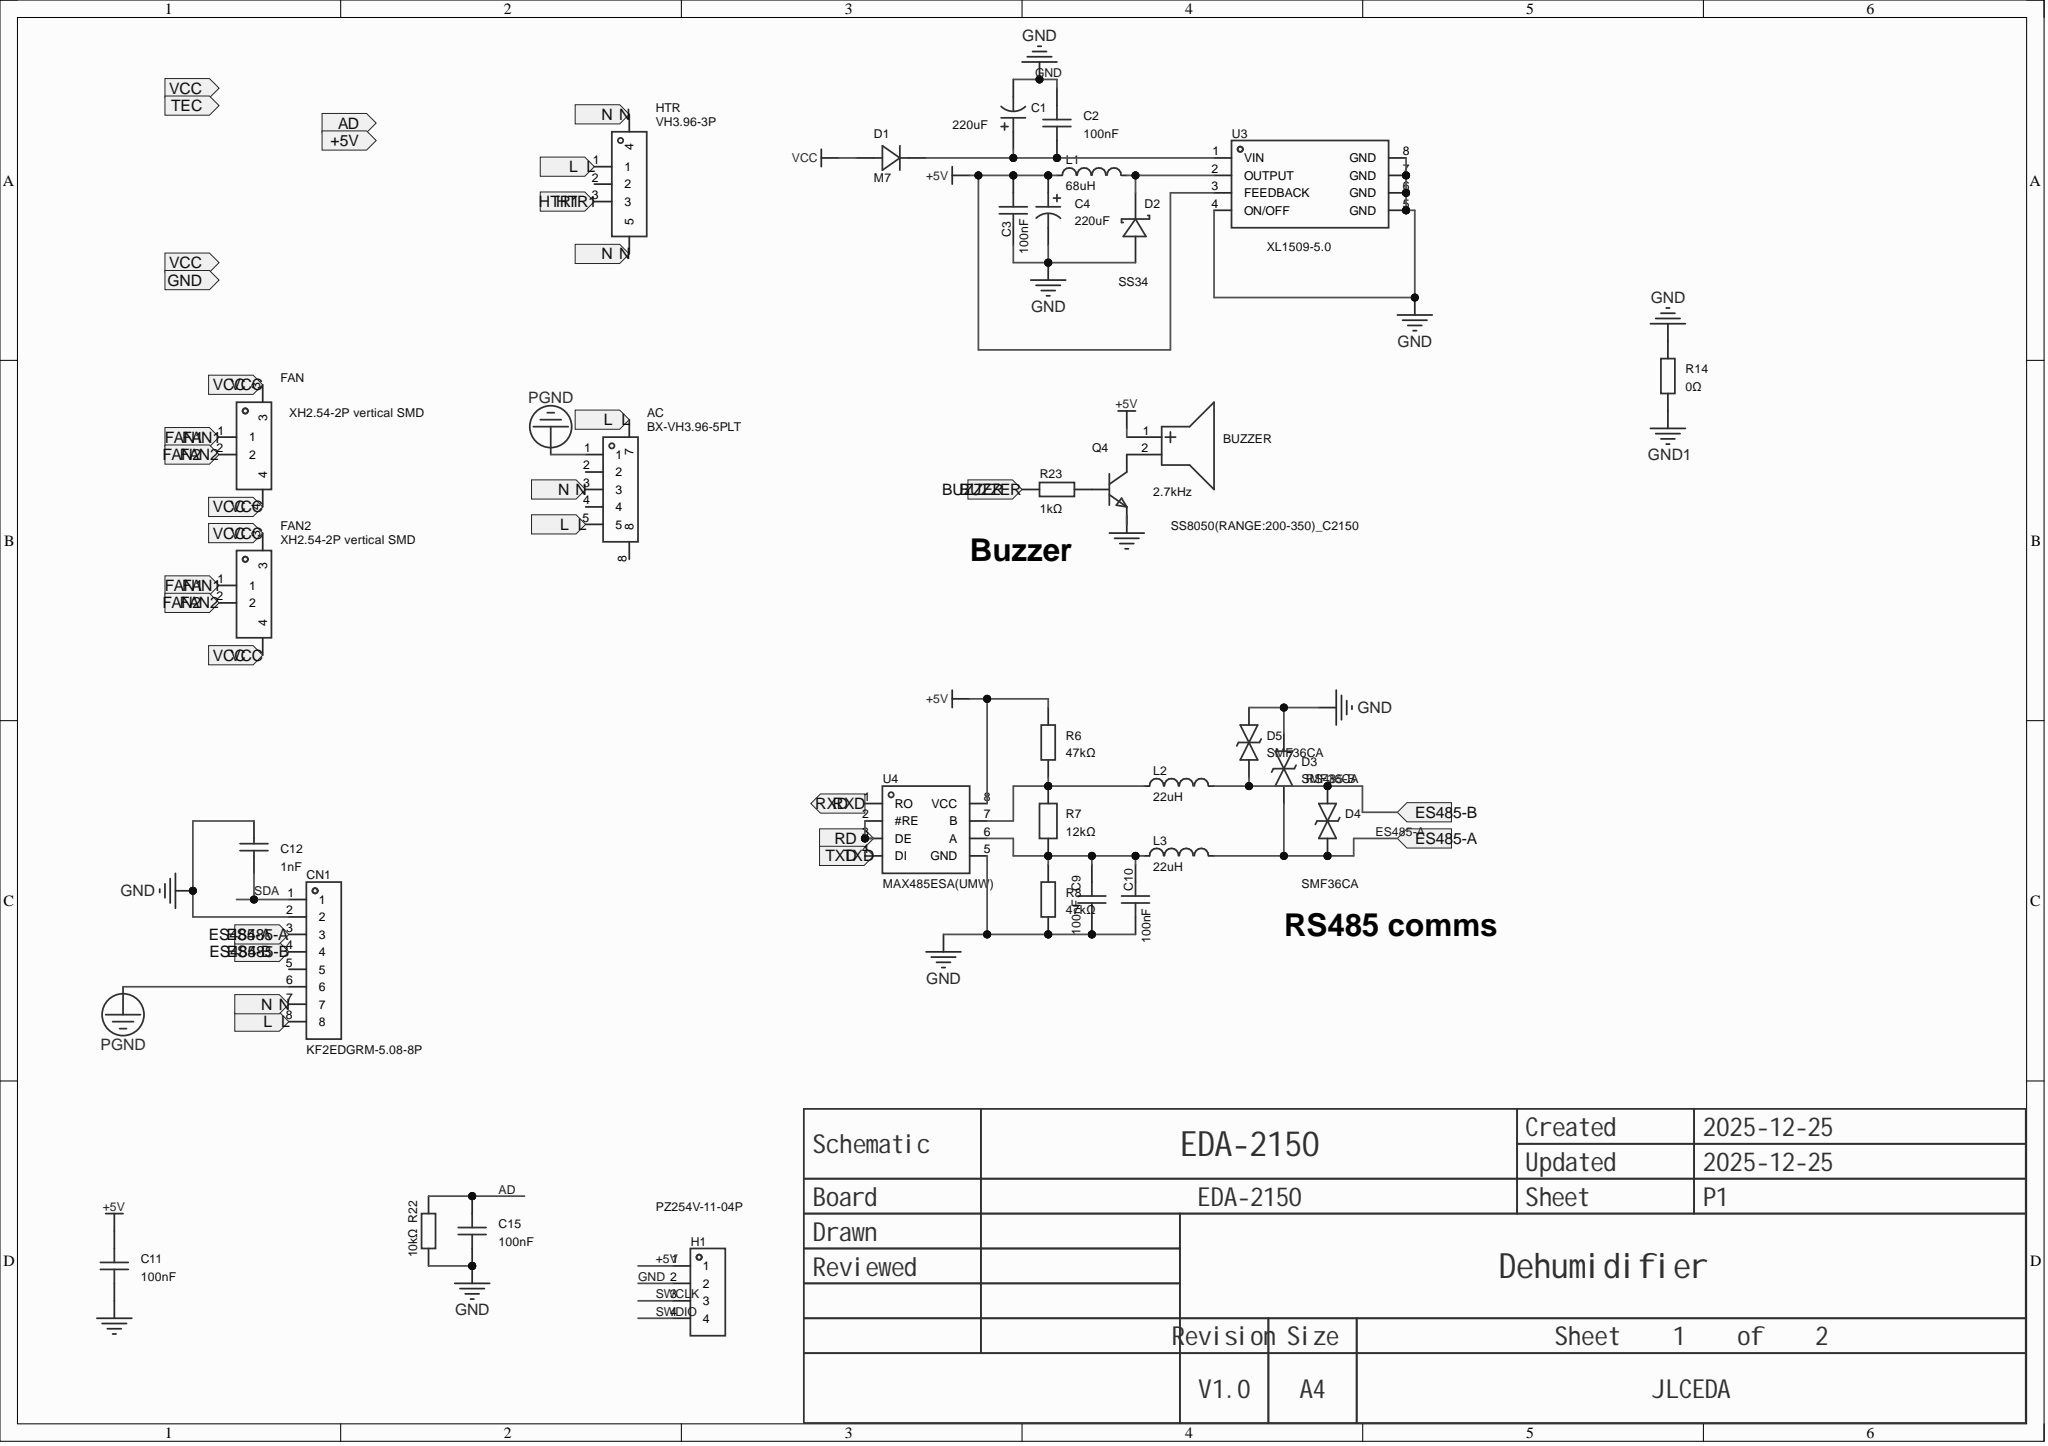Circuit board | Altium Designer | 76 parts | 60 nets
Bill of materials:
Comment,Description,Designator,Footprint,LibRef,Quantity
"BX-VH3.96-5PLT","Pin structure:1x5P;Pitch:3.96mm;Mounting:Vertical SMD;Series:VH;Total pins:5P;Rows:1;Pins per row:5;Row spacing:-;Rated current:7A;Contact material:Brass;Contact plating:Tin;Operating temp:-25℃~+85℃;","AC","CONN-SMD_5P-P3.96_BX-VH3.96-5PLT","BX-VH3.96-5PLT","1"
"2.7kHz","Drive:Active(built-in driver circuit);Frequency:2.7kHz;Sound pressure(SPL):80dB;","BUZZER","BUZ-SMD_L9.6-W9.6-LS10.0-R","YS-SBZ9650DYB05","1"
"220uF","Capacitance:220uF;Tolerance:±20%;Rated voltage:35V;Ripple current:190mA@120Hz;","C1, C4","CAP-SMD_BD6.3-L6.6-W6.6-FD","JVJ35V220M6x8","2"
"100nF","Capacitance:100nF;Tolerance:±10%;Rated voltage:50V;Temp coefficient:X7R;","C2, C3, C5, C9, C10, C11, C15, C16","C0805","FCC0805B104K500DT","8"
"100pF","Capacitance:100pF;Tolerance:±5%;Rated voltage:50V;Temp coefficient:C0G;","C6, C7, C8","C0805","CL21C101JBANNNC","3"
"1nF","Capacitance:1nF;Tolerance:±10%;Rated voltage:50V;Temp coefficient:X7R;","C12","C0805","CL21B102KBCNNNC","1"
"10nF","Capacitance:10nF;Tolerance:±10%;Rated voltage:50V;Temp coefficient:X7R;","C17","C1210","1210B103K500NT","1"
"KF2EDGRM-5.08-8P","Connector type:Board-side socket, closed;Fixing:Screw;Structure:1x8P;Pitch:5.08mm;Colour:Green;Mounting:Right-angle THT;Rows:1;Pins per row:8;Rated current:15A;Rated voltage:300V;Operating temp:-40℃~+105℃;","CN1","CONN-TH_8P-P5.08_KF2EDGRM-5.08-8P","KF2EDGRM-5.08-8P","1"
"M7","Diode configuration:1 single;Forward voltage(Vf):1.1V@1A;DC reverse voltage(Vr):1kV;Rectified current:1A;","D1","SMA_L4.4-W2.8-LS5.4-RD","M7_C46598121","1"
"SS34","Diode configuration:Single;Forward voltage(Vf):550mV@3A;DC reverse voltage(Vr):40V;Rectified current:3A;","D2, D6, D7","SMA_L4.3-W2.6-LS5.2-RD","SS34_C8678","3"
"SMF36CA","Polarity:Bidirectional;Reverse standoff voltage(Vrwm):36V;Clamping voltage:58.1V;Peak pulse current(Ipp):3.5A;Peak pulse power(Ppp):200W@10/1000us;Breakdown voltage:40V;","D3, D4, D5","SOD-123_L2.7-W1.8-LS3.7-BI","SMF36CA_C435502","3"
"XH2.54-2P vertical SMD","","FAN, FAN2","CONN-SMD_2P_A2501WV-S","XH2.54-2P立贴","2"
"PZ254V-11-04P","Pin structure:1x4P;Pitch:2.54mm;Row spacing:-;Round/square pin:Square pin;Mounting:Through-hole;Rows:Single row;Total pins:4P;Rated current:3A;Rated voltage:250V;Mating pin length:6mm;Body height:2.5mm;Tail length:3mm;Contact material:-;Operating temp:-40℃~+105℃;Colour:Black;","H1","HDR-TH_4P-P2.54-V-M","PZ254V-11-04P","1"
"VH3.96-3P","","HTR","CONN-SMD_3P-P3.96_HCTL_HC-VH-3ALT","VH3.96-3P","1"
"68uH","Inductance:68uH;Tolerance:±20%;Rated current:1.5A;Saturation current(Isat):2A;Type:-;","L1","IND-SMD_L7.1-W6.6_H5.0","PSPMAA0605H-680M-IGF","1"
"22uH","Inductance:22uH;Tolerance:±10%;Rated current:5mA;Saturation current(Isat):-;DC resistance(DCR):900mΩ;","L2, L3","L1206","SCL3216T220KSP","2"
"3mmFIR","","LED1, LED2, LED3, LED4","LED-TH_BD3.0-P2.54-FD","3mmFIR","4"
"SP420361N","Same display size as the 30V tester I bought, Digits:3 digits;Emitting colour:Red;LED polarity:Common cathode;Character height (inch):0.36;","LED5, LED6","LED-SEG-TH_SP420361N","EPHB_SP420361N 0.36英寸3位红色数码管","2"
"HYG140N10","Type:1 N-channel;Drain-source voltage(Vdss):100V;Continuous drain current(Id):45A;On-resistance(RDS(on)@Vgs,Id):-;Power(Pd):3W;Threshold voltage(Vgs(th)@Id):2.5V@250uA;","Q1","TO-252-3_L6.6-W6.1-P4.58-LS10.1-BR","NCE0140K2-VB","1"
"HYG025N06LS1B","Quantity:1 N-channel;Drain-source voltage(Vdss):60V;Continuous drain current(Id):160A;On-resistance(RDS(on)):3.3mΩ@10V;Power dissipation(Pd):125W;Threshold voltage(Vgs(th)):3V@250uA;","Q2","TO-263-2_L10.2-W8.7-P5.08-LS15.1-BR","HYG025N06LS1B","1"
"BTA216B-600D-JSM","Holding current(Ih):25mA;Off-state peak voltage(Vdrm):600V;Gate trigger current(Igt):50mA;","Q3","TO-263-3_L10.2-W9.2-P5.08-LS15.4-BR","BTA216B-600D-JSM","1"
"SS8050(RANGE:200-350)","Transistor type:NPN;Collector current(Ic):1.5A;C-E breakdown voltage(Vceo):25V;Power(Pd):300mW;DC current gain(hFE@Ic,Vce):200@800mA,1V;","Q4, Q5, Q6","SOT-23-3_L2.9-W1.3-P1.90-LS2.4-BR","SS8050(RANGE:200-350)_C2150","3"
"LBC807-25","Transistor type:PNP;Collector current(Ic):500mA;C-E breakdown voltage(Vceo):45V;Power(Pd):225mW;DC current gain(hFE@Ic,Vce):160@100mA,1.0V;","Q7","SOT-23-3_L2.9-W1.6-P1.90-LS2.8-BR","LBC807-25LT1G","1"
"1K","Resistor type:Thick film resistor;Resistance:1kΩ;Tolerance:±1%;Power:125mW;Max operating voltage:150V;Temp coefficient:±100ppm/?;","R1","R0805","0805W8F1001T5E","1"
"10kΩ","Resistor type:Thick film resistor;Resistance:1kΩ;Tolerance:±1%;Power:125mW;Max operating voltage:150V;Temp coefficient:±100ppm/?;, Resistor type:Thick film resistor;Resistance:10kΩ;Tolerance:±1%;Power:125mW;Operating voltage:150V;Temp coefficient:±100ppm/?;","R2, R3, R4, R5, R10, R17, R22","R0805","0805W8F1001T5E, 0805W8F1002T5E_C17414","7"
"47kΩ","Resistor type:Thick film resistor;Resistance:47kΩ;Tolerance:±1%;Power:125mW;Max operating voltage:150V;Temp coefficient:±100ppm/?;","R6, R8","R0805","0805W8F4702T5E","2"
"12kΩ","Resistor type:Thick film resistor;Resistance:12kΩ;Tolerance:±1%;Power:125mW;Operating voltage:150V;Temp coefficient:±100ppm/?;","R7","R0805","FRC0805F1202TS","1"
"10","","R9","R0805","Res_0805","1"
"1Ω","Resistor type:Thick film resistor;Resistance:1Ω;Tolerance:±1%;Power:250mW;Operating voltage:200V;Temp coefficient:±200ppm/?;","R11","R1206","FRC1206F1R00TS","1"
"1kΩ","Resistor type:Thick film resistor;Resistance:1kΩ;Tolerance:±1%;Power:125mW;Max operating voltage:150V;Temp coefficient:±100ppm/?;","R12, R16, R23","R0805","0805W8F1001T5E","3"
"47Ω","Resistance:47Ω;Tolerance:±0.5%;Temp coefficient:±25ppm/?;","R13","R0805","TRC0805D47R0P0525Z","1"
"0Ω","","R14","R0603","Res_0603","1"
"2.2kΩ","Resistor type:Thick film resistor;Resistance:2.2kΩ;Tolerance:±1%;Power:125mW;Operating voltage:150V;Temp coefficient:±100ppm/?;","R18","R0805","0805W8F2201T5E","1"
"51Ω","Resistor type:Thin film resistor;Resistance:51Ω;Tolerance:±1%;Power:400mW;Operating voltage:200V;Temp coefficient:±50ppm/?;","R19","R0204","MMA02040C5109FB300","1"
"150Ω","Resistor type:Thin film resistor;Resistance:150Ω;Tolerance:±0.1%;Power:250mW;Operating voltage:200V;Temp coefficient:±15ppm/?;","R20","R0204","MMA02040E1500BB100","1"
"120Ω","Resistance:120Ω;Tolerance:±1%;Power:250mW;Temp coefficient:±50ppm/?;","R21","R0204","CSR0204FTDV1200","1"
"1TS005F-2500-5001","Circuit:SPST;Button shape:Round button;Actuation force:2.5N;Mounting:Vertical SMD;Switch length:6mm;Switch width:6mm;Switch height:5mm;Bracket:Without bracket;Contact current:50mA;Rated voltage:12V;Lamp:None;Life:7 ten-thousand cycles;","SW1, SW2, SW3, SW4","SW-SMD_4P-L6.0-W6.0-P4.50-LS9.0-H2.5","1TS005F-2500-5001","4"
"TSSOP-20","","U1","TSSOP-20_L6.5-W4.4-P0.65-LS6.4-BL","LCM08F003","1"
"XL1509-5.0","Function:Buck;Output type:Fixed;Operating voltage:4.5V~40V;Output voltage:5V;Output current:2A;","U3","SOIC-8_L4.9-W3.9-P1.27-LS6.0-TR","XL1509-5.0","1"
"MAX485ESA(UMW)","","U4","SOP-8_L5.0-W4.0-P1.27-LS6.0-BL","MAX485ESA(UMW)","1"
"ELM3083(TA)-V","Forward voltage:1.5V;Forward current:60mA;Load voltage:800V;Static dv/dt:1000V/us;","U5","SOP-4_L4.4-W4.0-P2.54-LS7.0-TL","ELM3083(TA)-V","1"
"TM1668-SSOP24-TA2108","Type:-;Operating voltage(DC):3V~6V;Switching frequency:-;Channels:-;Output voltage:-;Output current:-;Dimming:-;Topology:-;","U6","SSOP-24_L8.1-W5.3-P0.65-LS7.8-BL","TM1668-SSOP24-TA2108","1"
Netlist (Protel format):
[
AC
CONN-SMD_5P-P3.96_BX-VH3.96-5PLT
BX-VH3.96-5PLT



]
[
BUZZER
BUZ-SMD_L9.6-W9.6-LS10.0-R
2.7kHz



]
[
C1
CAP-SMD_BD6.3-L6.6-W6.6-FD
220uF



]
[
C2
C0805
100nF



]
[
C3
C0805
100nF



]
[
C4
CAP-SMD_BD6.3-L6.6-W6.6-FD
220uF



]
[
C5
C0805
100nF



]
[
C6
C0805
100pF



]
[
C7
C0805
100pF



]
[
C8
C0805
100pF



]
[
C9
C0805
100nF



]
[
C10
C0805
100nF



]
[
C11
C0805
100nF



]
[
C12
C0805
1nF



]
[
C15
C0805
100nF



]
[
C16
C0805
100nF



]
[
C17
C1210
10nF



]
[
CN1
CONN-TH_8P-P5.08_KF2EDGRM-5.08-8P
KF2EDGRM-5.08-8P



]
[
D1
SMA_L4.4-W2.8-LS5.4-RD
M7



]
[
D2
SMA_L4.3-W2.6-LS5.2-RD
SS34



]
[
D3
SOD-123_L2.7-W1.8-LS3.7-BI
SMF36CA



]
[
D4
SOD-123_L2.7-W1.8-LS3.7-BI
SMF36CA



]
[
D5
SOD-123_L2.7-W1.8-LS3.7-BI
SMF36CA



]
[
D6
SMA_L4.3-W2.6-LS5.2-RD
SS34



]
[
D7
SMA_L4.3-W2.6-LS5.2-RD
SS34



]
[
FAN
CONN-SMD_2P_A2501WV-S
XH2.54-2P vertical SMD



]
[
FAN2
CONN-SMD_2P_A2501WV-S
XH2.54-2P vertical SMD



]
[
H1
HDR-TH_4P-P2.54-V-M
PZ254V-11-04P



]
[
HTR
CONN-SMD_3P-P3.96_HCTL_HC-VH-3ALT
VH3.96-3P



]
[
L1
IND-SMD_L7.1-W6.6_H5.0
68uH



]
[
L2
L1206
22uH



]
[
L3
L1206
22uH



]
[
LED1
LED-TH_BD3.0-P2.54-FD
3mmFIR



]
[
LED2
LED-TH_BD3.0-P2.54-FD
3mmFIR



]
[
LED3
LED-TH_BD3.0-P2.54-FD
3mmFIR



]
[
LED4
LED-TH_BD3.0-P2.54-FD
3mmFIR



]
[
LED5
LED-SEG-TH_SP420361N
SP420361N



]
[
LED6
LED-SEG-TH_SP420361N
SP420361N



]
[
Q1
TO-252-3_L6.6-W6.1-P4.58-LS10.1-BR
HYG140N10



]
[
Q2
TO-263-2_L10.2-W8.7-P5.08-LS15.1-BR
HYG025N06LS1B



]
[
Q3
TO-263-3_L10.2-W9.2-P5.08-LS15.4-BR
BTA216B-600D-JSM



]
[
Q4
SOT-23-3_L2.9-W1.3-P1.90-LS2.4-BR
SS8050(RANGE:200-350)



]
[
Q5
SOT-23-3_L2.9-W1.3-P1.90-LS2.4-BR
SS8050(RANGE:200-350)



]
[
Q6
SOT-23-3_L2.9-W1.3-P1.90-LS2.4-BR
SS8050(RANGE:200-350)



]
[
Q7
SOT-23-3_L2.9-W1.6-P1.90-LS2.8-BR
LBC807-25



]
[
R1
R0805
1K



]
[
R2
R0805
10kΩ



]
[
R3
R0805
10kΩ



]
[
R4
R0805
10kΩ



]
[
R5
R0805
10kΩ



]
[
R6
R0805
47kΩ



]
[
R7
R0805
12kΩ



]
[
R8
R0805
47kΩ



]
[
R9
R0805
10



]
[
R10
R0805
10kΩ



]
[
R11
R1206
1Ω



]
[
R12
R0805
1kΩ



]
[
R13
R0805
47Ω



]
[
R14
R0603
0Ω



]
[
R16
R0805
1kΩ



]
[
R17
R0805
10kΩ



]
[
R18
R0805
2.2kΩ



]
[
R19
R0204
51Ω



]
[
R20
R0204
150Ω



]
[
R21
R0204
120Ω



]
[
R22
R0805
10kΩ



]
[
R23
R0805
1kΩ



]
[
SW1
SW-SMD_4P-L6.0-W6.0-P4.50-LS9.0-H2.5
1TS005F-2500-5001



]
[
SW2
SW-SMD_4P-L6.0-W6.0-P4.50-LS9.0-H2.5
1TS005F-2500-5001



]
[
SW3
SW-SMD_4P-L6.0-W6.0-P4.50-LS9.0-H2.5
1TS005F-2500-5001



]
[
SW4
SW-SMD_4P-L6.0-W6.0-P4.50-LS9.0-H2.5
1TS005F-2500-5001



]
[
U1
TSSOP-20_L6.5-W4.4-P0.65-LS6.4-BL
TSSOP-20



]
[
U3
SOIC-8_L4.9-W3.9-P1.27-LS6.0-TR
XL1509-5.0



]
[
U4
SOP-8_L5.0-W4.0-P1.27-LS6.0-BL
MAX485ESA(UMW)



]
[
U5
SOP-4_L4.4-W4.0-P2.54-LS7.0-TL
ELM3083(TA)-V



]
[
U6
SSOP-24_L8.1-W5.3-P0.65-LS7.8-BL
TM1668-SSOP24-TA2108



]
(
TXD
U1-11
U4-4
)
(
SWDIO
H1-4
U1-8
)
(
SWCLK
H1-3
U1-18
)
(
STB
C6-2
R3-1
U1-17
U6-3
)
(
SDA
C12-1
CN1-1
R1-2
R2-1
)
(
RXD
U1-10
U4-1
)
(
PL
D6-2
Q2-4
)
(
PGND
AC-1
CN1-6
)
(
P
R12-1
U1-16
)
(
NetU4_2
U4-2
U4-3
)
(
NetR19_1
R19-1
U5-3
)
(
NetR18_1
R18-1
U5-1
)
(
NetR1_1
R1-1
U1-13
)
(
NetQ6_3
Q6-3
U5-2
)
(
NetQ6_1
Q6-1
R16-2
R17-1
)
(
NetQ5_3
Q5-3
R13-1
)
(
NetQ5_1
Q5-1
Q7-1
R12-2
)
(
NetQ4_1
Q4-1
R23-2
)
(
NetQ3_3
Q3-3
R19-2
R20-1
)
(
NetQ2_1
Q2-1
Q5-2
Q7-2
)
(
NetQ1_1
Q1-1
R9-2
R10-2
)
(
NetL2_1
L2-1
R6-1
R7-2
U4-7
)
(
NetD2_1
D2-1
L1-2
U3-2
)
(
NetC17_2
C17-2
R21-1
)
(
NetC9_2
C9-2
C10-2
L3-1
R7-1
R8-2
U4-6
)
(
NetC1_1
C1-1
C2-1
D1-1
U3-1
)
(
NetBUZZER_2
BUZZER-2
Q4-3
)
(
N
AC-3
C17-1
CN1-7
HTR-4
HTR-5
Q3-1
R20-2
)
(
L
AC-5
AC-7
CN1-8
HTR-1
)
(
KEY2
SW1-1
SW2-1
U6-5
)
(
KEY1
SW3-1
SW4-1
U6-4
)
(
HTR1
HTR-3
Q3-2
R21-2
U5-4
)
(
HTR
R16-1
U1-5
)
(
GND1
C16-1
Q2-3
Q6-2
Q7-3
R10-1
R11-1
R14-1
R17-2
)
(
GND
C1-2
C2-2
C3-1
C4-2
C5-2
C6-1
C7-1
C8-1
C9-1
C10-1
C11-1
C12-2
C15-1
CN1-2
D2-2
D3-2
D5-2
H1-2
Q4-2
R8-1
R14-2
R22-1
U1-7
U3-4
U3-5
U3-6
U3-7
U3-8
U4-5
U6-22
)
(
G
LED5-5
LED6-5
U6-13
)
(
FAN2
D1-2
D6-1
D7-1
FAN-2
FAN-3
FAN-4
FAN2-2
FAN2-3
FAN2-4
R18-2
)
(
FAN1
D7-2
FAN-1
FAN2-1
Q1-3
)
(
FAN
R9-1
U1-15
)
(
F
LED5-10
LED6-10
U6-12
)
(
ES485-B
CN1-4
D4-2
D5-1
L2-2
)
(
ES485-A
CN1-3
D3-1
D4-1
L3-2
)
(
E
LED5-1
LED6-1
U6-11
)
(
DP
LED5-3
LED6-3
U6-14
)
(
DIN
C8-2
R5-1
U1-6
U6-1
)
(
D
LED4-1
LED5-2
LED6-2
U6-10
)
(
CLK
C7-2
R4-1
U1-2
U6-2
)
(
C
LED3-1
LED5-4
LED6-4
U6-9
)
(
BUZZER
R23-1
U1-3
)
(
B
LED2-1
LED5-7
LED6-7
SW1-4
SW3-4
U6-8
)
(
AD5
C16-2
Q1-2
R11-2
U1-20
)
(
AD
C15-2
R22-2
U1-19
)
(
A
LED1-1
LED5-11
LED6-11
SW2-4
SW4-4
U6-7
)
(
+5V
BUZZER-1
C3-2
C4-1
C5-1
C11-2
H1-1
L1-1
R2-2
R3-2
R4-2
R5-2
R6-2
R13-2
U1-9
U3-3
U4-8
U6-6
)
(
7
LED1-2
LED2-2
LED3-2
LED4-2
U6-17
)
(
6
LED6-8
U6-18
)
(
4
LED6-12
U6-20
)
(
3
LED5-8
U6-21
)
(
2
LED5-9
U6-23
)
(
1
LED5-12
U6-24
)